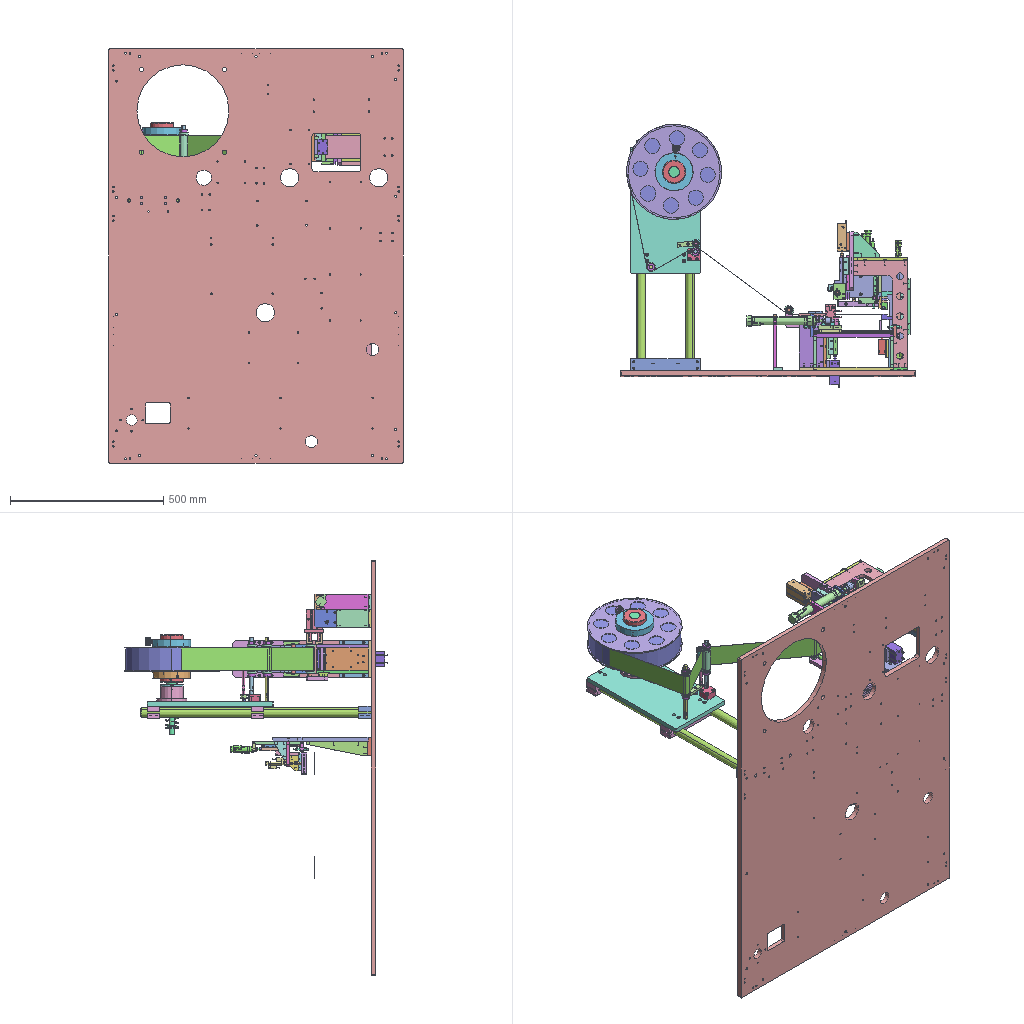Assembly | STEP file | 127 different items | 175 placed | box 960 x 858 x 1350 mm
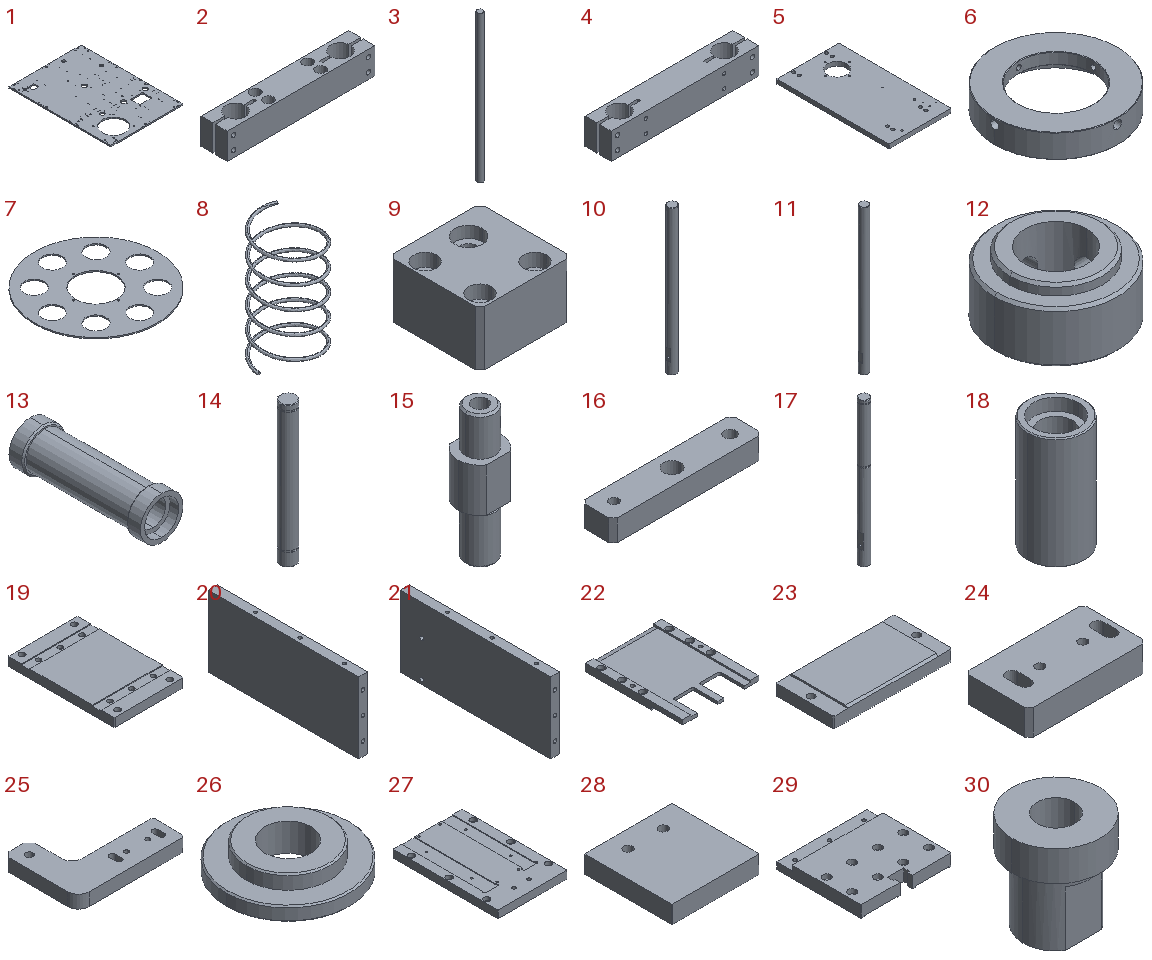Parts list (item | name | quantity | parent item | size | volume):
1 | 2001 Base plate | x1 | in 200 Bag feed section | 960 x 1350 x 16 mm | 18913226 mm3
2 | 2002 Support shaft connecting plate | x1 | in 200 Bag feed section | 226 x 40 x 40 mm | 266231 mm3
3 | 2003 Bag feed support shaft | x2 | in 200 Bag feed section | 30 x 30 x 750 mm | 528443 mm3
4 | 2004 Support shaft connecting plate A | x2 | in 200 Bag feed section | 226 x 40 x 40 mm | 281782 mm3
5 | 2005 Support shaft mounting plate | x1 | in 200 Bag feed section | 226 x 410 x 15 mm | 1321158 mm3
6 | 2006 Limit side plate B | x1 | in 200 Bag feed section | 125 x 125 x 24 mm | 134168 mm3
7 | 2007 Limit side plate A | x2 | in 200 Bag feed section | 310 x 310 x 3 mm | 153476 mm3
8 | 2002 Bag feed compression spring | x1 | in 200 Bag feed section | 42 x 42 x 80 mm | 2095 mm3
9 | 2008 Fixed block | x1 | in 200 Bag feed section | 40 x 40 x 24 mm | 33932 mm3
10 | 2009 Bag feed support shaft B | x1 | in 200 Bag feed section | 12 x 12 x 191 mm | 21066 mm3
11 | 2010 Bag feed support shaft | x1 | in 200 Bag feed section | 12 x 12 x 210 mm | 23133 mm3
12 | 2011 Stopper shaft | x4 | in 200 Bag feed section | 24 x 24 x 12 mm | 3483 mm3
13 | 2012 Guide shaft | x3 | in 200 Bag feed section | 30 x 92.5 x 30 mm | 26584 mm3
14 | 2013 Bag feed rotary shaft | x1 | in 200 Bag feed section | 12 x 12 x 108.5 mm | 11898 mm3
15 | 2014 Bag feed hold-down pivot shaft | x1 | in 200 Bag feed section | 12 x 10 x 36.5 mm | 2248 mm3
16 | 2015 Stopper | x1 | in 200 Bag feed section | 70 x 15 x 10 mm | 9229 mm3
17 | 2016 Hold-down material shaft | x1 | in 200 Bag feed section | 10 x 10 x 148 mm | 11241 mm3
18 | 2017 Hold-down shaft | x1 | in 200 Bag feed section | 28 x 28 x 55 mm | 20637 mm3
19 | 2018 Bag feed bottom plate 2 | x1 | in 200 Bag feed section | 80 x 122 x 10 mm | 91496 mm3
20 | 2019 Base support plate A | x1 | in 200 Bag feed section | 10 x 169 x 80 mm | 133994 mm3
21 | 2020 Base support plate B | x1 | in 200 Bag feed section | 10 x 169 x 80 mm | 131754 mm3
22 | 2021 Bottom plate | x1 | in 200 Bag feed section | 92 x 118 x 10 mm | 66642 mm3
23 | 2022 Hold-down plate | x1 | in 200 Bag feed section | 92 x 45 x 10 mm | 39337 mm3
24 | 2023 Pad plate | x1 | in 200 Bag feed section | 55 x 30 x 12 mm | 18040 mm3
25 | 2024 Bag feed rotary shaft mounting plate | x1 | in 200 Bag feed section | 100 x 70 x 12 mm | 44684 mm3
26 | 2025 Spring plate | x1 | in 200 Bag feed section | 44 x 44 x 10 mm | 8953 mm3
27 | 2026 Blade mounting base plate A | x1 | in 200 Bag feed section | 92 x 140 x 10 mm | 122641 mm3
28 | 2027 Cylinder pad block | x1 | in 200 Bag feed section | 50 x 50 x 10 mm | 24602 mm3
29 | 2028 Slider block connecting plate 1 | x1 | in 200 Bag feed section | 92 x 86 x 12 mm | 78738 mm3
30 | 2029 Bag feed cylinder joint | x2 | in 200 Bag feed section | 16 x 16 x 17.5 mm | 1737 mm3
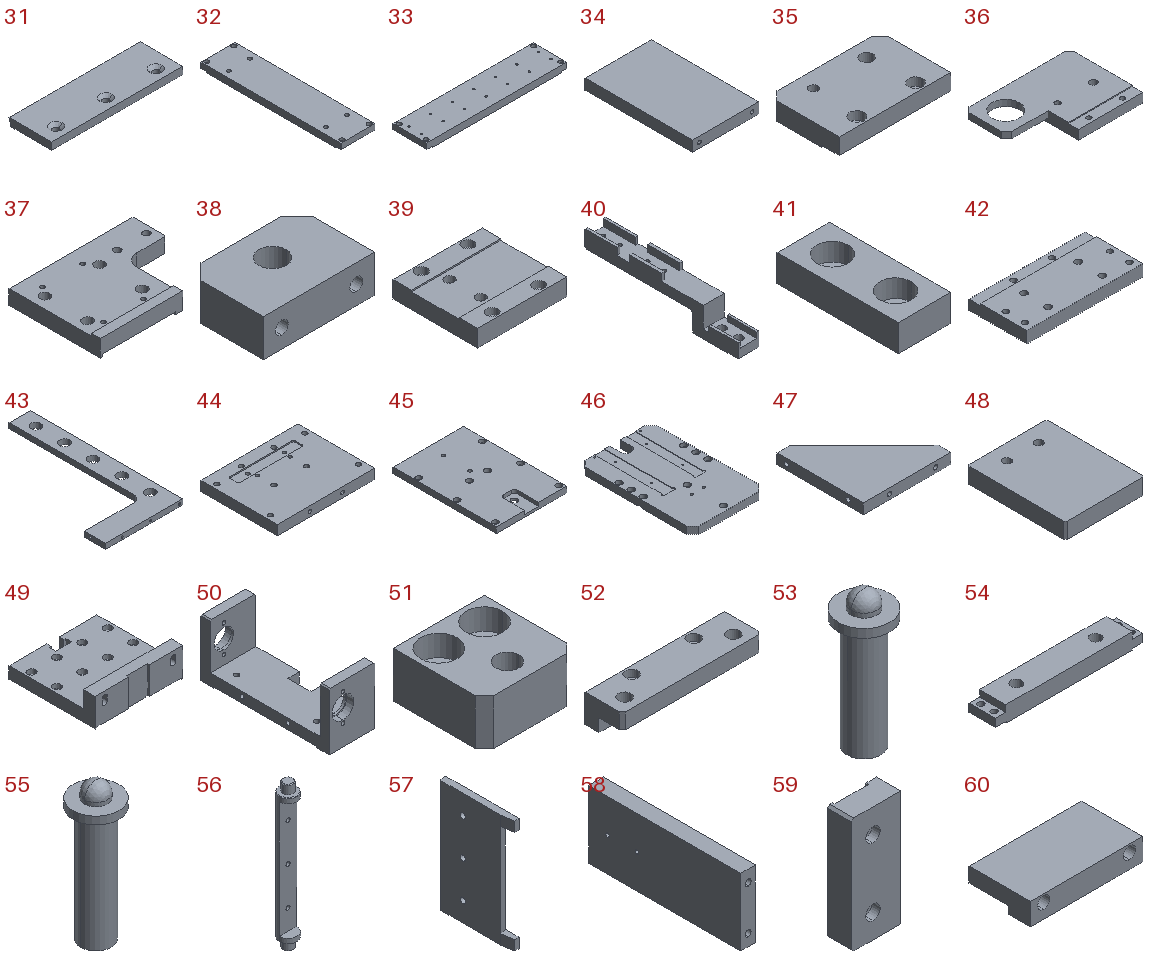31 | 2030 Blade A | x1 | in 200 Bag feed section | 92 x 30 x 5 mm | 13137 mm3
32 | 2031 Base bottom plate | x1 | in 200 Bag feed section | 63 x 260 x 12 mm | 191174 mm3
33 | 2032 Upper mounting plate on base | x1 | in 200 Bag feed section | 260 x 63 x 12 mm | 190964 mm3
34 | 2033 Reinforcing rib | x2 | in 200 Bag feed section | 63 x 102 x 10 mm | 63855 mm3
35 | 2034 Buffer mounting plate | x1 | in 200 Bag feed section | 63 x 40 x 10 mm | 23136 mm3
36 | 2035 Cylinder mounting seat 1 | x1 | in 200 Bag feed section | 103.5 x 72 x 10 mm | 50168 mm3
37 | 2036 Guide rail mounting plate | x1 | in 200 Bag feed section | 102 x 75 x 14 mm | 61484 mm3
38 | 2037 Bag feed mounting plate 3 | x1 | in 200 Bag feed section | 36 x 25 x 12 mm | 9371 mm3
39 | 2038 Bag feed cylinder mounting plate 12 | x1 | in 200 Bag feed section | 63 x 60 x 12 mm | 40268 mm3
40 | 2040 Cylinder material clamp B | x2 | in 200 Bag feed section | 15 x 110 x 25.8 mm | 13578 mm3
41 | 2041 Bag feed assist block | x4 | in 200 Bag feed section | 10 x 23 x 5.1 mm | 949.865 mm3
42 | 2042 Mounting base plate 3 | x1 | in 200 Bag feed section | 120 x 60 x 12 mm | 78438 mm3
43 | 2043 Reinforcing rib 2 | x2 | in 200 Bag feed section | 175 x 347 x 12 mm | 248598 mm3
44 | 2044 Support plate 2 | x1 | in 200 Bag feed section | 120 x 94 x 12 mm | 129518 mm3
45 | 2045 Upper plate | x1 | in 200 Bag feed section | 120 x 176 x 10 mm | 199306 mm3
46 | 2046 Upper blade mounting plate | x1 | in 200 Bag feed section | 120 x 190 x 12 mm | 255418 mm3
47 | 2047 Reinforcing rib 3 | x1 | in 200 Bag feed section | 85 x 84 x 10 mm | 44321 mm3
48 | 2048 Cylinder pad block B | x1 | in 200 Bag feed section | 50 x 62 x 10 mm | 30587 mm3
49 | 2049 Bag feed connecting plate 2 | x1 | in 200 Bag feed section | 90 x 88 x 29 mm | 100448 mm3
50 | 2050 Upper bearing mounting plate | x1 | in 200 Bag feed section | 40 x 112 x 50 mm | 59323 mm3
51 | 2051 Bag feed stopper block B | x1 | in 200 Bag feed section | 20 x 20 x 10 mm | 3129 mm3
52 | 2052 Spring mounting plate A | x1 | in 200 Bag feed section | 90 x 24 x 18 mm | 25874 mm3
53 | 2053 Spring mounting seat A | x2 | in 200 Bag feed section | 12 x 12 x 32 mm | 1418 mm3
54 | 2054 Buffer mounting seat | x1 | in 200 Bag feed section | 112 x 20 x 12 mm | 23091 mm3
55 | 2055 Spring mounting seat B | x2 | in 200 Bag feed section | 12 x 12 x 36 mm | 1619 mm3
56 | 2056 Blade rotary shaft | x1 | in 200 Bag feed section | 14 x 14 x 114 mm | 8821 mm3
57 | 2057 Bag feed blade B | x1 | in 200 Bag feed section | 5 x 60 x 92 mm | 22979 mm3
58 | 2058 Cylinder mounting plate | x1 | in 200 Bag feed section | 10 x 104 x 46 mm | 47342 mm3
59 | 2059 Cylinder press block A | x1 | in 200 Bag feed section | 20.5 x 10 x 48 mm | 8560 mm3
60 | 2060 Mounting plate | x1 | in 200 Bag feed section | 92 x 50 x 18 mm | 61462 mm3
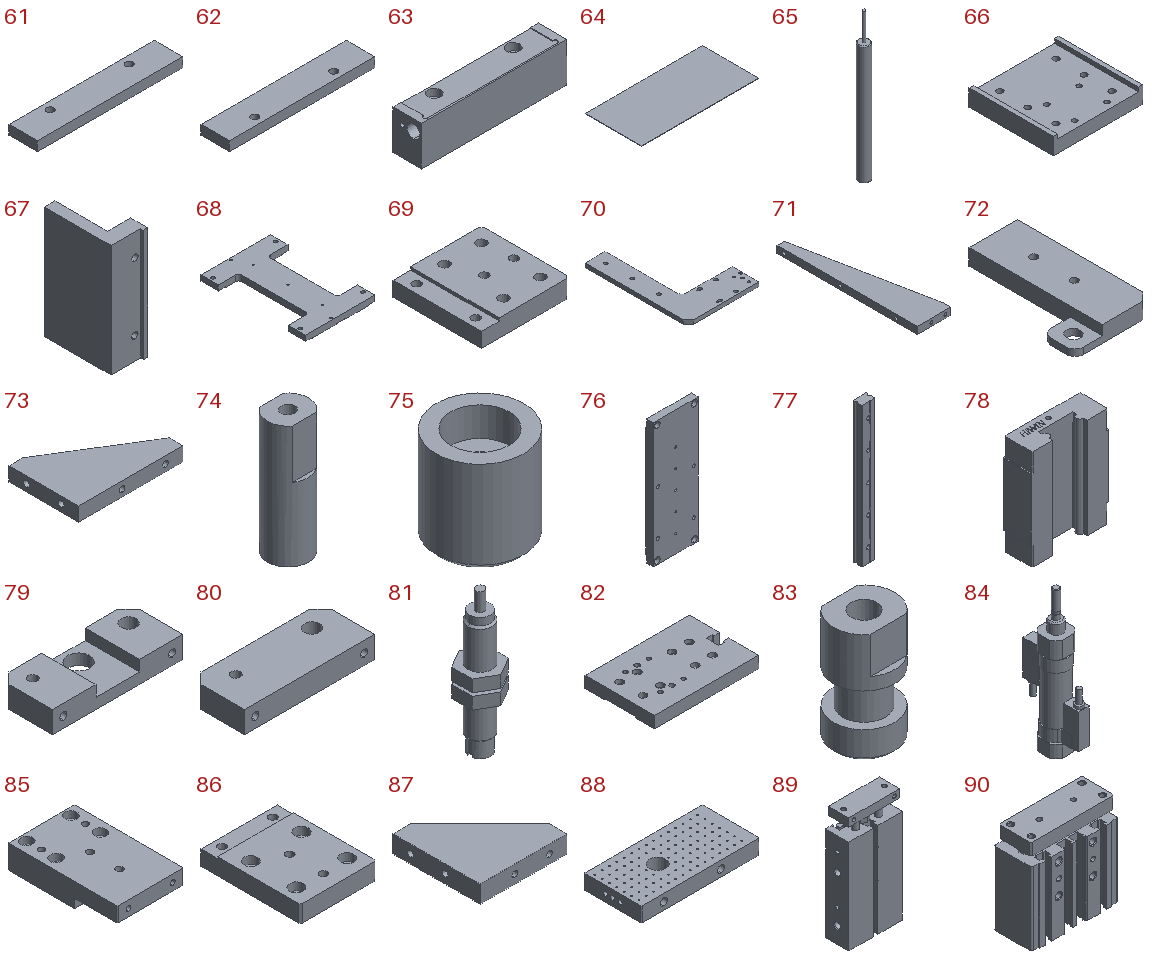61 | 2061 Bag feed artificial stone plate A | x2 | in 200 Bag feed section | 92 x 18 x 6 mm | 9745 mm3
62 | 2062 Pad plate | x1 | in 200 Bag feed section | 92 x 18 x 6 mm | 9745 mm3
63 | 2063 Heat press block A | x1 | in 200 Bag feed section | 92 x 18 x 25 mm | 33821 mm3
64 | Bag feed part 2 | x3 | in 200 Bag feed section | 150 x 72 x 0.5 mm | 5400 mm3
65 | 2064 Heating tube | x1 | in 200 Bag feed section | 8 x 8 x 106 mm | 4380 mm3
66 | 2065 Cylinder mounting plate 11 | x1 | in 200 Bag feed section | 64 x 60 x 12 mm | 34607 mm3
67 | 2066 Adapter plate | x1 | in 200 Bag feed section | 24 x 50 x 80 mm | 41824 mm3
68 | 2067 Gripper mounting plate | x1 | in 200 Bag feed section | 120 x 180 x 10 mm | 126941 mm3
69 | 2068 Support plate A base | x1 | in 200 Bag feed section | 60 x 60 x 12 mm | 37825 mm3
70 | 2069 Support plate B | x1 | in 200 Bag feed section | 212 x 310 x 12 mm | 361905 mm3
71 | 2070 Bag feed reinforcing rib 1 | x1 | in 200 Bag feed section | 48 x 200 x 10 mm | 58935 mm3
72 | 2071 Cylinder mounting plate 13 | x1 | in 200 Bag feed section | 47 x 82.5 x 10 mm | 24879 mm3
73 | 2072 Cylinder reinforcing rib plate | x1 | in 200 Bag feed section | 60 x 40 x 8 mm | 12139 mm3
74 | 2073 Stop shaft | x1 | in 200 Bag feed section | 10 x 10 x 30 mm | 2056 mm3
75 | 2074 Stop shaft 2 | x1 | in 200 Bag feed section | 15 x 15 x 16 mm | 2079 mm3
76 | 2075 Mounting base plate | x1 | in Bag feed mounting electronic clip AZ Z-axis | 60 x 10 x 167 mm | 95280 mm3
77 | Bag feed mounting electronic clip MGN12C (slide rail) Z-axis | x1 | in Bag feed mounting electronic clip AZ Z-axis | 12 x 8 x 125 mm | 10672 mm3
78 | Bag feed mounting electronic clip MGN12C (slider block) Z-axis | x2 | in Bag feed mounting electronic clip AZ Z-axis | 27 x 10 x 34.7 mm | 7013 mm3
79 | 2076 Cylinder mounting plate | x1 | in Bag feed mounting electronic clip AZ Z-axis | 60 x 25 x 10 mm | 11081 mm3
80 | 2077 Cylinder mounting plate | x1 | in Bag feed mounting electronic clip AZ Z-axis | 60 x 25 x 10 mm | 14024 mm3
81 | Bag feed mounting electronic clip RB0806Z Z-axis | x4 | in Bag feed mounting electronic clip AZ Z-axis, 200 Bag feed section | 12 x 13.856 x 46.8 mm | 2563 mm3
82 | 2078 Slider mounting plate | x1 | in Bag feed mounting electronic clip AZ Z-axis | 90 x 60 x 10 mm | 48995 mm3
83 | 2079 Bag feed floating joint mounting | x1 | in Bag feed mounting electronic clip AZ Z-axis | 10 x 10 x 18 mm | 891.186 mm3
84 | Bag feed cylinder CDJ2B16-30-C76 (0) | x1 | in Bag feed mounting electronic clip AZ Z-axis | 18.6 x 41.8 x 105 mm | 26186 mm3
85 | 2082 Bag feed connecting plate A | x1 | in Bag feed mounting electronic clip AZ Z-axis | 45 x 74 x 16 mm | 42322 mm3
86 | 2083 Bag feed connecting plate B | x1 | in Bag feed mounting electronic clip AZ Z-axis | 45 x 59 x 10 mm | 23585 mm3
87 | 2084 Bag feed suction plate reinforcement | x1 | in 200 Bag feed section | 50 x 50 x 10 mm | 16595 mm3
88 | 2085 Upper suction plate | x1 | in 200 Bag feed section | 145 x 70 x 18 mm | 152195 mm3
89 | Bag feed cylinder CXSM6-20-Z76L (0) | x1 | in 200 Bag feed section | 37 x 16.2 x 78.5 mm | 36756 mm3
90 | Bag feed cylinder MGPM12-20-Z76L (0) | x1 | in 200 Bag feed section | 58 x 26 x 62 mm | 70641 mm3
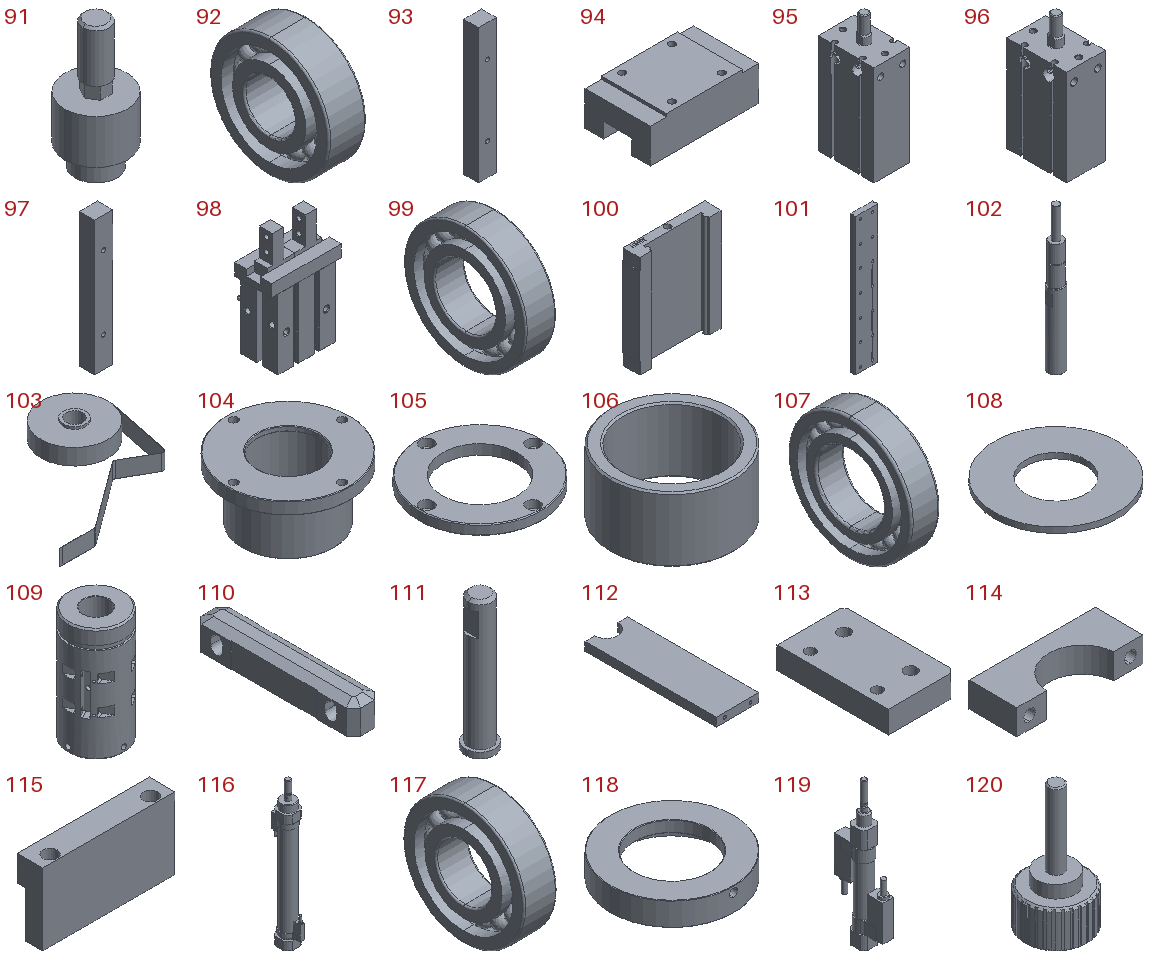91 | Bag feed JA30-10-125 floating joint | x1 | in 200 Bag feed section | 24 x 24 x 49.5 mm | 10590 mm3
92 | deep groove ball bearings gb_Rolling bearings 619-8 GB 276-94 | x2 | in 200 Bag feed section | 6 x 19 x 19 mm | 1029 mm3
93 | Bag feed EGH15SA guide rail | x2 | in 200 Bag feed section | 15 x 12.5 x 114 mm | 21017 mm3
94 | Bag feed EGH15CA slider | x6 | in 200 Bag feed section | 56.8 x 34 x 19.5 mm | 29571 mm3
95 | Bag feed cylinder CDU25-40D-A93L (0) | x1 | in 200 Bag feed section | 32 x 50 x 122 mm | 135464 mm3
96 | Bag feed cylinder CDU25-30D-A93L (0) | x1 | in 200 Bag feed section | 32 x 50 x 112 mm | 120089 mm3
97 | Bag feed guide rail | x2 | in 200 Bag feed section | 15 x 12.5 x 110 mm | 20267 mm3
98 | Bag feed finger cylinder MHZ2-25D-F8N (19.3) | x1 | in 200 Bag feed section | 63 x 52.1 x 102.7 mm | 124711 mm3
99 | deep groove ball bearings gb_Rolling bearings 61901 GB 276-94 | x6 | in 200 Bag feed section | 6 x 24 x 24 mm | 1508 mm3
100 | Bag feed MGW15H slider | x1 | in 200 Bag feed section | 60 x 12.6 x 73.8 mm | 36057 mm3
101 | Bag feed MGW15H slide rail | x1 | in 200 Bag feed section | 42 x 9.5 x 257 mm | 96343 mm3
102 | 2086 Fixed shaft | x1 | in 200 Bag feed section | 35 x 35 x 325.3 mm | 236741 mm3
103 | Transparent bag feed part | x1 | in 200 Bag feed section | 682 x 614 x 93 mm | 4868515 mm3
104 | 2087 Bag feed material shaft A | x1 | in 200 Bag feed section | 100 x 100 x 50 mm | 131531 mm3
105 | 2088 Bag feed shaft end cap | x1 | in 200 Bag feed section | 74 x 74 x 6 mm | 15191 mm3
106 | 2097 Shaft bearing | x1 | in 200 Bag feed section | 38 x 38 x 20 mm | 8302 mm3
107 | deep groove ball bearings gb_Rolling bearings 6006 GB 276-94 | x2 | in 200 Bag feed section | 13 x 55 x 55 mm | 16022 mm3
108 | 2089 Compression block A | x1 | in 200 Bag feed section | 66 x 66 x 3 mm | 7851 mm3
109 | 2090 Fixed material shaft | x1 | in 200 Bag feed section | 76 x 76 x 154 mm | 511727 mm3
110 | 2091 Clamp block | x3 | in 200 Bag feed section | 10 x 56 x 10 mm | 4506 mm3
111 | 2092 Shaft | x6 | in 200 Bag feed section | 5 x 5 x 23 mm | 291.029 mm3
112 | 2095 Cylinder support plate | x1 | in 200 Bag feed section | 50 x 153 x 10 mm | 73275 mm3
113 | 2094 Cylinder support base plate | x1 | in 200 Bag feed section | 30 x 50 x 10 mm | 13851 mm3
114 | 2096 Bag feed cylinder support plate B | x1 | in 200 Bag feed section | 50 x 19 x 10 mm | 6027 mm3
115 | 2081 Heat lower plate | x1 | in 200 Bag feed section | 92 x 18 x 50 mm | 61665 mm3
116 | Bag feed cylinder CDM2BZ25-150-C73 (0) | x1 | in 200 Bag feed section | 30 x 52.6 x 257 mm | 140263 mm3
117 | deep groove ball bearings gb_Rolling bearings 61900 GB 276-94 | x2 | in 200 Bag feed section | 6 x 22 x 22 mm | 1339 mm3
118 | 2093 Limit side plate B2 | x1 | in 200 Bag feed section | 125 x 125 x 24 mm | 136649 mm3
119 | Cylinder CDJ2B10-30-C73 (0) | x1 | in 200 Bag feed section | 12.2 x 35.4 x 104 mm | 14245 mm3
120 | M6 Bag feed screw | x1 | in 200 Bag feed section | 25 x 24.98 x 50 mm | 8815 mm3
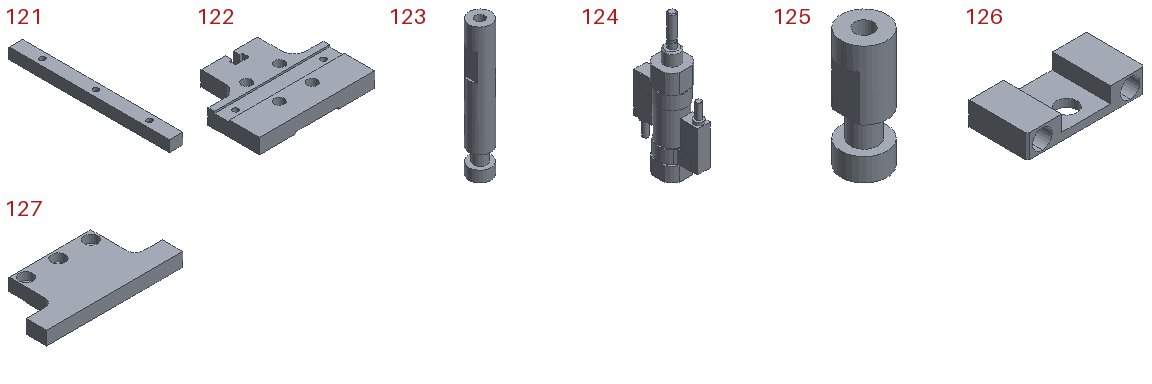121 | Guide rail | x1 | in 200 Bag feed section | 15 x 180 x 12.5 mm | 33214 mm3
122 | 2098 Connecting plate A | x2 | in 200 Bag feed section | 92 x 70 x 12 mm | 53453 mm3
123 | 2101 Cylinder joint B | x1 | in 200 Bag feed section | 10 x 10 x 61 mm | 4191 mm3
124 | Cylinder CDJ2B16-15-C73 (0) | x2 | in 200 Bag feed section | 18.6 x 41.8 x 90 mm | 22619 mm3
125 | 2100 Cylinder joint | x1 | in 200 Bag feed section | 10 x 10 x 26 mm | 1459 mm3
126 | 2099 Cylinder mounting plate | x1 | in 200 Bag feed section | 60 x 30 x 12 mm | 12721 mm3
127 | 006 | x1 | in 200 Bag feed section | 80 x 38 x 8 mm | 16678 mm3
Placements (level | parent | child | x y z in mm | rotation matrix by rows):
1 | 200 Bag feed section | 2001 Base plate | 480.0 -16.0 -675.0 | 1 0 0 0 0 1 0 -1 0
1 | 200 Bag feed section | 2002 Support shaft connecting plate | 146.0 0.0 -494.0 | 1 0 0 0 0 1 0 -1 0
1 | 200 Bag feed section | 2003 Bag feed support shaft | 66.0 -0.0 -494.0 | 0.698 -0.7161 0 0 0 1 -0.7161 -0.698 0
1 | 200 Bag feed section | 2003 Bag feed support shaft | 226.0 -0.0 -494.0 | -0.4615 -0.8872 0 0 0 1 -0.8872 0.4615 0
1 | 200 Bag feed section | 2004 Support shaft connecting plate A | 146.0 349.0 -494.0 | 1 0 0 0 0 1 0 -1 0
1 | 200 Bag feed section | 2004 Support shaft connecting plate A | 146.0 689.0 -494.0 | 1 0 0 0 0 1 0 -1 0
1 | 200 Bag feed section | 2005 Support shaft mounting plate | 146.0 524.0 -474.0 | 1 0 0 0 1 0 0 0 1
1 | 200 Bag feed section | 2006 Limit side plate B | 174.0 649.0 -356.0 | -0.9534 -0.3017 0 -0.3017 0.9534 0 0 0 -1
1 | 200 Bag feed section | 2007 Limit side plate A | 174.0 649.0 -356.0 | 0.4608 0.8875 0 0.8875 -0.4608 0 0 0 -1
1 | 200 Bag feed section | 2002 Bag feed compression spring | 174.0 649.0 -542.0 | 0.163 -0.9866 0 0.9866 0.163 0 0 0 1
1 | 200 Bag feed section | 2008 Fixed block | 239.0 379.0 -459.0 | 1 0 0 0 1 0 0 0 1
1 | 200 Bag feed section | 2009 Bag feed support shaft B | 244.0 389.0 -440.0 | -0.3304 0.9438 0 -0.9438 -0.3304 0 0 0 1
1 | 200 Bag feed section | 2010 Bag feed support shaft | 99.0 339.0 -459.0 | -0.9251 0.3797 0 -0.3797 -0.9251 0 0 0 1
1 | 200 Bag feed section | 2011 Stopper shaft | 99.0 339.0 -378.15 | 1 0 0 0 1 0 0 0 1
1 | 200 Bag feed section | 2012 Guide shaft | 99.0 339.0 -273.75 | -0.5679 0 -0.8231 0.8231 0 -0.5679 0 -1 -0
1 | 200 Bag feed section | 2012 Guide shaft | 549.0 198.5 -273.75 | -0.8241 0 -0.5665 0.5665 0 -0.8241 0 -1 -0
1 | 200 Bag feed section | 2013 Bag feed rotary shaft | 549.0 198.5 -366.363 | 0.6721 -0.7405 0 0.7405 0.6721 0 0 0 1
1 | 200 Bag feed section | 2014 Bag feed hold-down pivot shaft | 219.0 414.0 -459.0 | 0.9523 0.3053 0 -0.3053 0.9523 0 0 0 1
1 | 200 Bag feed section | 2015 Stopper | 219.0 414.0 -447.0 | 0.9974 -0.07151 0 0.07151 0.9974 0 0 0 1
1 | 200 Bag feed section | 2016 Hold-down material shaft | 245.931 415.931 -437.0 | 1 0 0 0 1 0 0 0 1
1 | 200 Bag feed section | 2017 Hold-down shaft | 245.931 415.931 -347.9 | 1 0 0 0 1 0 0 0 1
1 | 200 Bag feed section | 2018 Bag feed bottom plate 2 | 622.0 0.0 -320.0 | 1 0 0 0 0 1 0 -1 0
1 | 200 Bag feed section | 2019 Base support plate A | 582.0 93.5 -279.0 | 0 0 1 0 1 0 -1 0 -0
1 | 200 Bag feed section | 2020 Base support plate B | 582.0 93.5 -361.0 | 0 0 1 0 1 0 -1 0 0
1 | 200 Bag feed section | 2021 Bottom plate | 641.0 177.0 -320.0 | 0 -1 0 0 0 1 -1 0 0
1 | 200 Bag feed section | 2022 Hold-down plate | 634.5 195.5 -320.0 | 0 -1 0 0 0 -1 1 0 0
1 | 200 Bag feed section | 2023 Pad plate | 609.5 155.5 -377.464 | -1 0 0 0 -1 0 0 0 1
1 | 200 Bag feed section | 2024 Bag feed rotary shaft mounting plate | 587.0 175.5 -389.464 | 1 0 0 0 1 0 0 0 1
1 | 200 Bag feed section | 2025 Spring plate | 174.0 649.0 -547.0 | 1 0 0 0 1 0 0 0 1
1 | 200 Bag feed section | 2026 Blade mounting base plate A | 662.0 80.0 -320.0 | 0 0 1 0 1 0 -1 0 -0
1 | 200 Bag feed section | 2027 Cylinder pad block | 672.0 10.0 -320.0 | 0 0 1 0 1 0 -1 0 -0
1 | 200 Bag feed section | 2028 Slider block connecting plate 1 | 694.0 97.5 -320.0 | 0 0 1 0 1 0 -1 0 -0
1 | 200 Bag feed section | 2029 Bag feed cylinder joint | 698.0 48.0 -320.0 | -0.9237 0.383 0 0 0 1 0.383 0.9237 0
1 | 200 Bag feed section | 2029 Bag feed cylinder joint | 721.0 378.0 -320.0 | 1 0 0 0 0 -1 0 1 0
1 | 200 Bag feed section | 2030 Blade A | 701.0 139.5 -320.0 | 0 0 1 0 1 0 -1 0 -0
1 | 200 Bag feed section | 2031 Base bottom plate | 758.5 12.0 -185.3 | 0 1 0 0 0 -1 -1 0 -0
1 | 200 Bag feed section | 2032 Upper mounting plate on base | 758.5 110.0 -185.3 | 1 0 0 0 0 1 0 -1 0
1 | 200 Bag feed section | 2033 Reinforcing rib | 878.5 10.0 -153.8 | 0 0 1 0 1 0 -1 0 -0
1 | 200 Bag feed section | 2033 Reinforcing rib | 628.5 10.0 -153.8 | 0 0 1 0 1 0 -1 0 -0
1 | 200 Bag feed section | 2034 Buffer mounting plate | 887.5 132.0 -185.3 | 0 0 1 0 1 0 -1 0 -0
1 | 200 Bag feed section | 2035 Cylinder mounting seat 1 | 619.5 148.0 -165.05 | 0 0 1 0 1 0 -1 0 -0
1 | 200 Bag feed section | 2036 Guide rail mounting plate | 683.5 136.0 -166.3 | 0 1 0 0 0 1 1 0 0
1 | 200 Bag feed section | 2037 Bag feed mounting plate 3 | 710.0 160.5 -133.3 | 0 0 -1 0 1 0 1 0 0
1 | 200 Bag feed section | 2038 Bag feed cylinder mounting plate 12 | 683.5 148.0 -185.8 | 0 1 0 0 0 1 1 0 0
1 | 200 Bag feed section | 2040 Cylinder material clamp B | 683.5 210.65 -292.5 | -1 0 0 0 0 -1 0 -1 -0
1 | 200 Bag feed section | 2040 Cylinder material clamp B | 683.5 159.35 -292.5 | 1 0 0 0 0 1 0 -1 0
1 | 200 Bag feed section | 2041 Bag feed assist block | 683.5 189.85 -304.0 | 1 0 0 0 0 -1 0 1 -0
1 | 200 Bag feed section | 2042 Mounting base plate 3 | 904.0 0.0 -320.0 | 0 -1 0 0 0 1 -1 0 -0
1 | 200 Bag feed section | 2043 Reinforcing rib 2 | 886.0 359.0 -260.0 | 1 0 0 0 -1 0 0 0 -1
1 | 200 Bag feed section | 2043 Reinforcing rib 2 | 886.0 359.0 -368.0 | 1 0 0 0 -1 0 0 0 -1
1 | 200 Bag feed section | 2044 Support plate 2 | 874.0 57.0 -320.0 | 0 0 1 0 1 0 -1 0 0
1 | 200 Bag feed section | 2045 Upper plate | 846.0 359.0 -320.0 | 0 -1 0 0 0 1 -1 0 -0
1 | 200 Bag feed section | 2046 Upper blade mounting plate | 759.0 358.0 -320.0 | 0 0 -1 0 -1 0 -1 0 -0
1 | 200 Bag feed section | 2047 Reinforcing rib 3 | 759.0 369.0 -325.0 | 1 0 0 0 1 0 0 0 1
1 | 200 Bag feed section | 2048 Cylinder pad block B | 747.0 422.0 -320.0 | 0 0 -1 0 -1 0 -1 0 0
1 | 200 Bag feed section | 2049 Bag feed connecting plate 2 | 725.0 327.5 -320.0 | 0 0 -1 0 1 0 1 0 0
1 | 200 Bag feed section | 2050 Upper bearing mounting plate | 714.0 284.5 -320.0 | 1 0 0 0 0 -1 0 1 0
1 | 200 Bag feed section | 2051 Bag feed stopper block B | 724.0 274.5 -320.0 | 0 0 1 0 1 0 -1 0 -0
1 | 200 Bag feed section | 2052 Spring mounting plate A | 694.0 271.5 -320.0 | 0 0 -1 0 1 0 1 0 0
1 | 200 Bag feed section | 2053 Spring mounting seat A | 702.0 268.0 -285.0 | 0 0 1 -0.385 -0.9229 0 0.9229 -0.385 -0
1 | 200 Bag feed section | 2054 Buffer mounting seat | 733.0 244.5 -320.0 | 0 0 1 0 1 0 -1 0 0
1 | 200 Bag feed section | 2055 Spring mounting seat B | 715.0 244.5 -290.0 | 0 0 -1 0.2923 0.9563 0 0.9563 -0.2923 0
1 | 200 Bag feed section | 2056 Blade rotary shaft | 706.0 254.5 -370.0 | 0 -1 0 1 0 0 0 0 1
1 | 200 Bag feed section | 2057 Bag feed blade B | 708.5 243.5 -366.0 | 1 0 0 0 1 0 0 0 1
1 | 200 Bag feed section | 2058 Cylinder mounting plate | 843.5 307.0 -297.0 | 1 0 0 0 -1 0 0 0 -1
1 | 200 Bag feed section | 2059 Cylinder press block A | 835.5 223.5 -356.0 | 1 0 0 0 1 0 0 0 1
1 | 200 Bag feed section | 2060 Mounting plate | 860.0 242.5 -320.0 | 0 1 0 0 0 1 1 0 -0
1 | 200 Bag feed section | 2061 Bag feed artificial stone plate A | 860.0 242.5 -320.0 | 0 1 0 0 0 -1 -1 0 0
1 | 200 Bag feed section | 2061 Bag feed artificial stone plate A | 860.0 230.5 -320.0 | 0 1 0 0 0 -1 -1 0 0
1 | 200 Bag feed section | 2062 Pad plate | 860.0 230.5 -320.0 | 0 -1 0 0 0 1 -1 0 -0
1 | 200 Bag feed section | 2063 Heat press block A | 860.0 224.5 -320.0 | 0 1 0 0 0 -1 -1 0 0
1 | 200 Bag feed section | Bag feed part 2 | 781.0 185.0 -320.0 | 1 0 0 0 0 1 0 -1 -0
1 | 200 Bag feed section | 2064 Heating tube | 856.0 206.5 -280.0 | -0.9539 -0.3001 0 -0.3001 0.9539 0 0 0 -1
1 | 200 Bag feed section | 2065 Cylinder mounting plate 11 | 874.0 74.0 -320.0 | 0 0 -1 0 -1 0 -1 0 0
1 | 200 Bag feed section | 2066 Adapter plate | 854.0 140.0 -360.0 | 1 0 0 0 1 0 0 0 1
1 | 200 Bag feed section | 2067 Gripper mounting plate | 933.0 210.0 -320.0 | 0 0 1 0 1 0 -1 0 0
1 | 200 Bag feed section | Bag feed part 2 | 781.0 185.0 -660.0 | 1 0 0 0 0 1 0 -1 -0
1 | 200 Bag feed section | Bag feed part 2 | 781.0 185.0 -1000.0 | 1 0 0 0 0 1 0 -1 -0
1 | 200 Bag feed section | 2068 Support plate A base | 905.0 0.0 -605.5 | 0 -1 0 0 0 1 -1 0 -0
1 | 200 Bag feed section | 2069 Support plate B | 905.0 165.0 -587.5 | -1 0 0 0 -1 0 0 0 1
1 | 200 Bag feed section | 2070 Bag feed reinforcing rib 1 | 900.0 12.0 -587.5 | 0 0 1 0 1 0 -1 0 0
1 | 200 Bag feed section | 2071 Cylinder mounting plate 13 | 746.5 265.0 -628.75 | -1 0 0 0 0 1 0 1 -0
1 | 200 Bag feed section | 2072 Cylinder reinforcing rib plate | 734.0 275.0 -587.5 | 0 0 1 0 1 0 -1 0 -0
1 | 200 Bag feed section | 2073 Stop shaft | 761.0 221.0 -660.0 | 1 0 0 0 0 1 0 -1 -0
1 | 200 Bag feed section | 2074 Stop shaft 2 | 761.0 210.0 -660.0 | 0.6993 -0.7149 0 0 0 1 -0.7149 -0.6993 -0
1 | 200 Bag feed section | Bag feed mounting electronic clip AZ Z-axis | 806.144 120.0 -590.635 | 1 0 0 0 0 1 0 -1 -0
2 | Bag feed mounting electronic clip AZ Z-axis | 2075 Mounting base plate | -0.1435 1.865 100.0 | 1 0 0 0 1 0 0 0 1
2 | Bag feed mounting electronic clip AZ Z-axis | Bag feed mounting electronic clip MGN12C (slide rail) Z-axis | -0.1435 5.865 149.0 | 1 0 0 0 1 0 0 0 1
2 | Bag feed mounting electronic clip AZ Z-axis | Bag feed mounting electronic clip MGN12C (slider block) Z-axis | -0.1435 5.865 208.5 | 1 0 0 0 1 0 0 0 1
2 | Bag feed mounting electronic clip AZ Z-axis | 2076 Cylinder mounting plate | -0.1435 18.365 257.0 | 1 0 0 0 1 0 0 0 1
2 | Bag feed mounting electronic clip AZ Z-axis | 2077 Cylinder mounting plate | -0.1435 18.365 100.0 | 1 0 0 0 1 0 0 0 1
2 | Bag feed mounting electronic clip AZ Z-axis | Bag feed mounting electronic clip RB0806Z Z-axis | 21.857 22.865 237.6 | -0.9783 0.2073 0 0.2073 0.9783 0 0 0 -1
2 | Bag feed mounting electronic clip AZ Z-axis | Bag feed mounting electronic clip MGN12C (slider block) Z-axis | -0.1435 5.865 163.5 | 1 0 0 0 1 0 0 0 1
2 | Bag feed mounting electronic clip AZ Z-axis | 2078 Slider mounting plate | -0.1435 17.865 186.0 | 0 1 0 0 0 1 1 0 0
2 | Bag feed mounting electronic clip AZ Z-axis | 2079 Bag feed floating joint mounting | -0.1435 23.865 226.0 | 0.9974 0.0727 0 -0.0727 0.9974 0 0 0 1
2 | Bag feed mounting electronic clip AZ Z-axis | Bag feed cylinder CDJ2B16-30-C76 (0) | -0.1435 23.865 254.0 | -0.4007 0.9162 0 0.9162 0.4007 0 0 0 -1
2 | Bag feed mounting electronic clip AZ Z-axis | 2082 Bag feed connecting plate A | -0.1435 27.865 154.0 | -1 0 0 0 0 1 0 1 0
2 | Bag feed mounting electronic clip AZ Z-axis | 2083 Bag feed connecting plate B | -0.1435 63.365 108.0 | -1 0 0 0 -1 0 0 0 1
1 | 200 Bag feed section | 2084 Bag feed suction plate reinforcement | 801.0 238.0 -634.5 | 0 0 1 0 1 0 -1 0 -0
1 | 200 Bag feed section | 2085 Upper suction plate | 778.5 228.0 -660.0 | 1 0 0 0 0 -1 0 1 0
1 | 200 Bag feed section | Bag feed cylinder CXSM6-20-Z76L (0) | 822.5 255.0 -320.0 | 0 1 0 0 0 -1 -1 0 -0
1 | 200 Bag feed section | Bag feed cylinder MGPM12-20-Z76L (0) | 852.0 104.0 -320.0 | 0 -1 0 0 0 1 -1 0 -0
1 | 200 Bag feed section | Bag feed JA30-10-125 floating joint | 658.5 163.0 -133.3 | 0 0 1 0.619 0.7854 0 -0.7854 0.619 -0
1 | 200 Bag feed section | deep groove ball bearings gb_Rolling bearings 619-8 GB 276-94 | 706.0 254.5 -267.0 | 0 0.09076 -0.9959 0 0.9959 0.09076 1 0 -0
1 | 200 Bag feed section | deep groove ball bearings gb_Rolling bearings 619-8 GB 276-94 | 706.0 254.5 -373.0 | 0 -0.09171 0.9958 0 0.9958 0.09171 -1 0 -0
1 | 200 Bag feed section | 2055 Spring mounting seat B | 715.0 244.5 -350.0 | 0 0 -1 0.2923 0.9563 0 0.9563 -0.2923 0
1 | 200 Bag feed section | Bag feed EGH15SA guide rail | 741.75 377.0 -346.0 | 0 -1 0 0 0 -1 1 0 -0
1 | 200 Bag feed section | Bag feed EGH15SA guide rail | 741.75 377.0 -294.0 | 0 -1 0 0 0 -1 1 0 -0
1 | 200 Bag feed section | Bag feed EGH15CA slider | 743.5 341.5 -346.0 | 0 0 -1 1 0 0 0 -1 -0
1 | 200 Bag feed section | Bag feed EGH15CA slider | 743.5 341.5 -294.0 | 0 0 -1 1 0 0 0 -1 -0
1 | 200 Bag feed section | Bag feed cylinder CDU25-40D-A93L (0) | 721.0 391.0 -320.0 | 1 0 0 0 0 -1 0 1 0
1 | 200 Bag feed section | Bag feed cylinder CDU25-30D-A93L (0) | 698.0 35.0 -320.0 | 1 0 0 0 0 1 0 -1 0
1 | 200 Bag feed section | Bag feed guide rail | 677.25 40.0 -346.0 | 0 1 0 0 0 1 1 0 -0
1 | 200 Bag feed section | Bag feed EGH15CA slider | 675.5 83.5 -346.0 | 0 0 1 1 0 0 0 1 0
1 | 200 Bag feed section | Bag feed guide rail | 677.25 40.0 -294.0 | 0 1 0 0 0 1 1 0 0
1 | 200 Bag feed section | Bag feed EGH15CA slider | 675.5 83.5 -294.0 | 0 0 1 1 0 0 0 1 -0
1 | 200 Bag feed section | 2053 Spring mounting seat A | 702.0 268.0 -355.0 | 0 0 1 -0.4265 -0.9045 0 0.9045 -0.4265 -0
1 | 200 Bag feed section | 2041 Bag feed assist block | 683.5 189.85 -336.0 | 1 0 0 0 0 -1 0 1 -0
1 | 200 Bag feed section | 2041 Bag feed assist block | 683.5 180.15 -304.0 | 1 0 0 0 0 1 0 -1 0
1 | 200 Bag feed section | 2041 Bag feed assist block | 683.5 180.15 -336.0 | -1 0 0 0 0 1 0 1 0
1 | 200 Bag feed section | Bag feed mounting electronic clip RB0806Z Z-axis | 634.9 144.0 -200.05 | 0 0 1 -0.9716 -0.2365 0 0.2365 -0.9716 -0
1 | 200 Bag feed section | Bag feed mounting electronic clip RB0806Z Z-axis | 874.1 143.0 -200.3 | 0 0 -1 -0.6061 0.7954 0 0.7954 0.6061 0
1 | 200 Bag feed section | 2011 Stopper shaft | 244.0 389.0 -378.15 | 0.624 0.7814 0 -0.7814 0.624 0 0 0 1
1 | 200 Bag feed section | 2012 Guide shaft | 244.0 389.0 -273.75 | -0.516 0 -0.8566 0.8566 0 -0.516 0 -1 -0
1 | 200 Bag feed section | Bag feed finger cylinder MHZ2-25D-F8N (19.3) | 683.5 185.0 -234.4 | 0 1 0 1 0 0 0 0 -1
1 | 200 Bag feed section | deep groove ball bearings gb_Rolling bearings 61901 GB 276-94 | 99.0 339.0 -276.85 | 0 0 1 0 1 0 -1 0 -0
1 | 200 Bag feed section | deep groove ball bearings gb_Rolling bearings 61901 GB 276-94 | 244.0 389.0 -363.15 | 0 0 1 0 1 0 -1 0 -0
1 | 200 Bag feed section | deep groove ball bearings gb_Rolling bearings 61901 GB 276-94 | 99.0 339.0 -363.15 | 0 0.1016 0.9948 0 0.9948 -0.1016 -1 0 -0
1 | 200 Bag feed section | deep groove ball bearings gb_Rolling bearings 61901 GB 276-94 | 244.0 389.0 -276.85 | 0 0 1 0 1 0 -1 0 -0
1 | 200 Bag feed section | 2011 Stopper shaft | 99.0 339.0 -261.85 | -0.3966 -0.918 0 -0.918 0.3966 0 0 0 -1
1 | 200 Bag feed section | 2011 Stopper shaft | 244.0 389.0 -261.85 | -0.7555 -0.6551 0 -0.6551 0.7555 0 0 0 -1
1 | 200 Bag feed section | deep groove ball bearings gb_Rolling bearings 61901 GB 276-94 | 549.0 198.5 -363.15 | 0 0 1 0 1 0 -1 0 -0
1 | 200 Bag feed section | deep groove ball bearings gb_Rolling bearings 61901 GB 276-94 | 549.0 198.5 -276.85 | 0 0 1 0 1 0 -1 0 -0
1 | 200 Bag feed section | Bag feed MGW15H slider | 683.5 122.0 -185.3 | 0 0 -1 0 1 0 1 0 -0
1 | 200 Bag feed section | Bag feed MGW15H slide rail | 887.0 122.0 -185.3 | 0 0 -1 0 1 0 1 0 -0
1 | 200 Bag feed section | 2086 Fixed shaft | 174.0 649.0 -409.0 | -0.4335 -0.9012 0 -0.9012 0.4335 0 0 0 -1
1 | 200 Bag feed section | 2007 Limit side plate A | 174.0 649.0 -284.0 | 0.7666 -0.6421 0 0.6421 0.7666 0 0 0 1
1 | 200 Bag feed section | Transparent bag feed part | 174.0 649.0 -320.0 | -1 0 0 0 1 0 0 0 -1
1 | 200 Bag feed section | 2087 Bag feed material shaft A | 174.0 649.0 -409.0 | -1 0 0 0 1 0 0 0 -1
1 | 200 Bag feed section | 2088 Bag feed shaft end cap | 174.0 649.0 -409.0 | 1 0 0 0 1 0 0 0 1
1 | 200 Bag feed section | 2097 Shaft bearing | 174.0 649.0 -422.0 | -0.8981 0.4399 0 0.4399 0.8981 0 0 0 -1
1 | 200 Bag feed section | deep groove ball bearings gb_Rolling bearings 6006 GB 276-94 | 174.0 649.0 -415.5 | 0 0.4399 0.8981 0 0.8981 -0.4399 -1 0 0
1 | 200 Bag feed section | deep groove ball bearings gb_Rolling bearings 6006 GB 276-94 | 174.0 649.0 -448.5 | 0 0.4399 0.8981 0 0.8981 -0.4399 -1 0 0
1 | 200 Bag feed section | 2089 Compression block A | 174.0 649.0 -462.0 | 1 -0.001375 0 0.001375 1 0 0 0 1
1 | 200 Bag feed section | 2090 Fixed material shaft | 174.0 649.0 -395.0 | 0.9965 0.08307 0 -0.08307 0.9965 0 0 0 1
1 | 200 Bag feed section | 2091 Clamp block | 176.402 677.816 -319.0 | 0.9965 0 0.08307 -0.08307 0 0.9965 0 -1 -0
1 | 200 Bag feed section | 2092 Shaft | 188.7 680.889 -339.0 | 0.006901 0.08278 -0.9965 0.08278 0.9931 0.08307 0.9965 -0.08307 0
1 | 200 Bag feed section | 2092 Shaft | 188.7 680.889 -299.0 | 0.006901 0.08278 -0.9965 0.08278 0.9931 0.08307 0.9965 -0.08307 0
1 | 200 Bag feed section | 2092 Shaft | 194.267 620.325 -339.0 | 0.06824 0.8187 0.5702 -0.04737 -0.5682 0.8215 0.9965 -0.08307 0
1 | 200 Bag feed section | 2092 Shaft | 194.267 620.325 -299.0 | 0.06824 0.8187 0.5702 -0.04737 -0.5682 0.8215 0.9965 -0.08307 0
1 | 200 Bag feed section | 2091 Clamp block | 197.754 632.512 -319.0 | -0.5702 0 0.8215 -0.8215 0 -0.5702 0 -1 0
1 | 200 Bag feed section | 2095 Cylinder support plate | 498.5 86.5 -133.3 | 0 0 1 0 1 0 -1 0 0
1 | 200 Bag feed section | 2094 Cylinder support base plate | 513.5 0.0 -133.3 | 1 0 0 0 0 1 0 -1 0
1 | 200 Bag feed section | 2096 Bag feed cylinder support plate B | 498.5 173.0 -133.3 | 0 0 1 0 1 0 -1 0 -0
1 | 200 Bag feed section | Bag feed mounting electronic clip RB0806Z Z-axis | 824.0 245.4 -613.5 | -0.5974 0.802 0 0 0 1 0.802 0.5974 -0
1 | 200 Bag feed section | 2092 Shaft | 139.033 645.786 -339.0 | -0.07514 -0.9014 0.4263 -0.03542 -0.4249 -0.9046 0.9965 -0.08307 0
1 | 200 Bag feed section | 2092 Shaft | 139.033 645.786 -299.0 | -0.07514 -0.9014 0.4263 -0.03542 -0.4249 -0.9046 0.9965 -0.08307 0
1 | 200 Bag feed section | 2091 Clamp block | 147.844 636.672 -319.0 | -0.4263 0 -0.9046 0.9046 0 -0.4263 0 -1 -0
1 | 200 Bag feed section | 2081 Heat lower plate | 869.0 176.0 -320.0 | 0 0 -1 0 1 0 1 0 0
1 | 200 Bag feed section | Bag feed cylinder CDM2BZ25-150-C73 (0) | 636.5 163.0 -133.3 | 0 0 1 -0.8704 0.4923 0 -0.4923 -0.8704 -0
1 | 200 Bag feed section | deep groove ball bearings gb_Rolling bearings 61900 GB 276-94 | 245.931 415.931 -295.9 | 0 0 1 0 1 0 -1 0 0
1 | 200 Bag feed section | deep groove ball bearings gb_Rolling bearings 61900 GB 276-94 | 245.931 415.931 -344.9 | 0 0 1 0 1 0 -1 0 0
1 | 200 Bag feed section | 2093 Limit side plate B2 | 174.0 649.0 -284.0 | -0.9961 -0.08808 0 0.08808 -0.9961 0 0 0 1
1 | 200 Bag feed section | Cylinder CDJ2B10-30-C73 (0) | 761.0 261.0 -660.0 | 1 0 0 0 0 -1 0 1 -0
1 | 200 Bag feed section | M6 Bag feed screw | 181.53 734.168 -263.0 | 0.9922 -0.08773 -0.08808 -0.08773 0.007757 -0.9961 0.08808 0.9961 -0
1 | 200 Bag feed section | Bag feed EGH15CA slider | 929.5 173.0 -320.0 | 0 0 -1 1 0 0 0 -1 -0
1 | 200 Bag feed section | Guide rail | 934.0 210.0 -320.0 | 0 0 -1 0 1 0 1 0 -0
1 | 200 Bag feed section | Bag feed EGH15CA slider | 929.5 254.5 -320.0 | 0 0 -1 1 0 0 0 -1 -0
1 | 200 Bag feed section | 2098 Connecting plate A | 911.5 259.5 -320.0 | 0 0 -1 0 1 0 1 0 -0
1 | 200 Bag feed section | 2101 Cylinder joint B | 904.5 284.0 -320.0 | 0.9999 0.01222 0 0 0 1 0.01222 -0.9999 -0
1 | 200 Bag feed section | Cylinder CDJ2B16-15-C73 (0) | 904.5 355.0 -320.0 | 0.9897 -0.1434 0 0 0 -1 0.1434 0.9897 0
1 | 200 Bag feed section | 2098 Connecting plate A | 911.5 168.0 -320.0 | 0 0 -1 0 -1 0 -1 0 -0
1 | 200 Bag feed section | 2100 Cylinder joint | 904.5 129.5 -320.0 | 0.8376 0.5463 0 0 0 -1 -0.5463 0.8376 0
1 | 200 Bag feed section | Cylinder CDJ2B16-15-C73 (0) | 904.5 93.5 -320.0 | -0.6489 0.7609 0 0 0 1 0.7609 0.6489 -0
1 | 200 Bag feed section | 2099 Cylinder mounting plate | 899.5 89.5 -320.0 | 0 -1 0 0 0 -1 1 0 -0
1 | 200 Bag feed section | 006 | 841.5 223.5 -320.0 | 0 0 1 0 1 0 -1 0 0